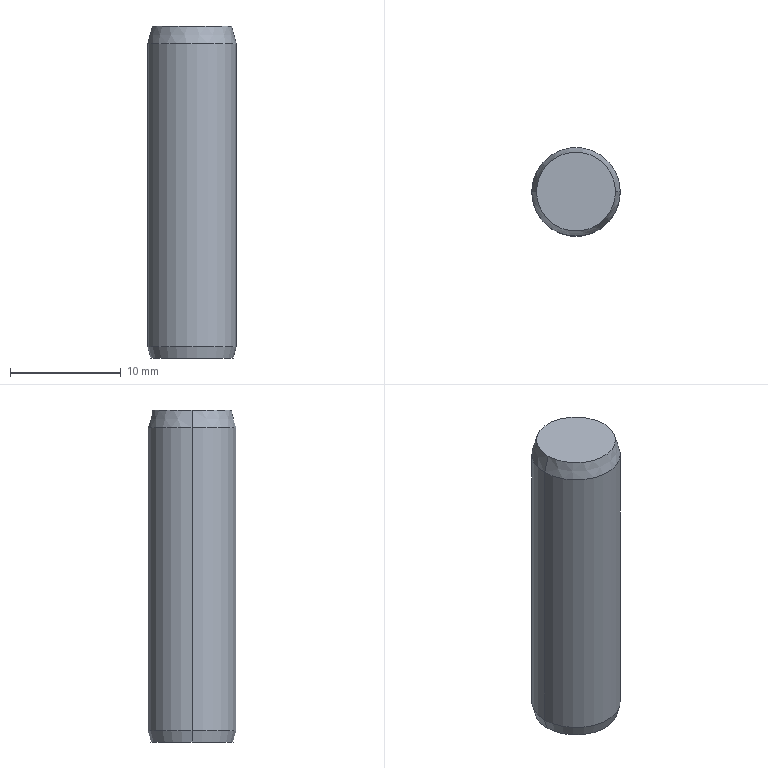Part | SolidWorks | features Chamfer 3, Cut 2, Extrusion 1, RevCut 1 | 1 solid | 16 faces | box 8 x 8 x 30 mm | volume 1303 mm3 | cone 8 | cylinder 6 | plane 2 | commonest cylinder face diameters 4.33 x2 5.3 x2 8 x2
STEP:
#1=CARTESIAN_POINT('',(2.165,0.,1.685));
#2=VERTEX_POINT('',#1);
#3=CARTESIAN_POINT('',(-2.165,0.,1.685));
#4=VERTEX_POINT('',#3);
#5=CARTESIAN_POINT('',(0.,0.,1.685));
#6=DIRECTION('',(0.,0.,-1.));
#7=DIRECTION('',(-1.,0.,0.));
#8=AXIS2_PLACEMENT_3D('',#5,#6,#7);
#9=CIRCLE('',#8,2.165);
#10=EDGE_CURVE('',#2,#4,#9,.T.);
#11=ORIENTED_EDGE('',*,*,#10,.F.);
#12=CARTESIAN_POINT('',(2.65,0.,1.2));
#13=VERTEX_POINT('',#12);
#14=CARTESIAN_POINT('',(2.65,0.,1.2));
#15=DIRECTION('',(0.7071,0.,-0.7071));
#16=VECTOR('',#15,1000.);
#17=LINE('',#14,#16);
#18=EDGE_CURVE('',#2,#13,#17,.T.);
#19=ORIENTED_EDGE('',*,*,#18,.T.);
#20=CARTESIAN_POINT('',(-2.65,0.,1.2));
#21=VERTEX_POINT('',#20);
#22=CARTESIAN_POINT('',(0.,0.,1.2));
#23=DIRECTION('',(0.,0.,-1.));
#24=DIRECTION('',(-1.,0.,0.));
#25=AXIS2_PLACEMENT_3D('',#22,#23,#24);
#26=CIRCLE('',#25,2.65);
#27=EDGE_CURVE('',#13,#21,#26,.T.);
#28=ORIENTED_EDGE('',*,*,#27,.T.);
#29=CARTESIAN_POINT('',(-2.65,0.,1.2));
#30=DIRECTION('',(-0.7071,0.,-0.7071));
#31=VECTOR('',#30,1000.);
#32=LINE('',#29,#31);
#33=EDGE_CURVE('',#4,#21,#32,.T.);
#34=ORIENTED_EDGE('',*,*,#33,.F.);
#35=EDGE_LOOP('',(#11,#19,#28,#34));
#36=FACE_OUTER_BOUND('',#35,.T.);
#37=CARTESIAN_POINT('',(0.,0.,1.2));
#38=DIRECTION('',(0.,0.,-1.));
#39=DIRECTION('',(-1.,0.,0.));
#40=AXIS2_PLACEMENT_3D('',#37,#38,#39);
#41=CONICAL_SURFACE('',#40,2.65,0.7854);
#42=ADVANCED_FACE('',(#36),#41,.F.);
#43=CARTESIAN_POINT('',(-2.165,0.,12.));
#44=VERTEX_POINT('',#43);
#45=CARTESIAN_POINT('',(2.165,0.,12.));
#46=VERTEX_POINT('',#45);
#47=CARTESIAN_POINT('',(0.,0.,12.));
#48=DIRECTION('',(0.,0.,1.));
#49=DIRECTION('',(1.,0.,0.));
#50=AXIS2_PLACEMENT_3D('',#47,#48,#49);
#51=CIRCLE('',#50,2.165);
#52=EDGE_CURVE('',#44,#46,#51,.T.);
#53=ORIENTED_EDGE('',*,*,#52,.T.);
#54=CARTESIAN_POINT('',(2.165,0.,12.));
#55=DIRECTION('',(0.,0.,-1.));
#56=VECTOR('',#55,1000.);
#57=LINE('',#54,#56);
#58=EDGE_CURVE('',#46,#2,#57,.T.);
#59=ORIENTED_EDGE('',*,*,#58,.T.);
#60=ORIENTED_EDGE('',*,*,#10,.T.);
#61=CARTESIAN_POINT('',(-2.165,0.,12.));
#62=DIRECTION('',(0.,0.,-1.));
#63=VECTOR('',#62,1000.);
#64=LINE('',#61,#63);
#65=EDGE_CURVE('',#44,#4,#64,.T.);
#66=ORIENTED_EDGE('',*,*,#65,.F.);
#67=EDGE_LOOP('',(#53,#59,#60,#66));
#68=FACE_OUTER_BOUND('',#67,.T.);
#69=CARTESIAN_POINT('',(0.,0.,12.));
#70=DIRECTION('',(0.,0.,-1.));
#71=DIRECTION('',(-1.,0.,0.));
#72=AXIS2_PLACEMENT_3D('',#69,#70,#71);
#73=CYLINDRICAL_SURFACE('',#72,2.165);
#74=ADVANCED_FACE('',(#68),#73,.F.);
#75=CARTESIAN_POINT('',(0.,0.,13.25));
#76=VERTEX_POINT('',#75);
#77=CARTESIAN_POINT('',(-2.165,0.,12.));
#78=DIRECTION('',(-0.866,0.,-0.5));
#79=VECTOR('',#78,1000.);
#80=LINE('',#77,#79);
#81=EDGE_CURVE('',#76,#44,#80,.T.);
#82=ORIENTED_EDGE('',*,*,#81,.F.);
#83=CARTESIAN_POINT('',(2.165,0.,12.));
#84=DIRECTION('',(0.866,0.,-0.5));
#85=VECTOR('',#84,1000.);
#86=LINE('',#83,#85);
#87=EDGE_CURVE('',#76,#46,#86,.T.);
#88=ORIENTED_EDGE('',*,*,#87,.T.);
#89=ORIENTED_EDGE('',*,*,#52,.F.);
#90=EDGE_LOOP('',(#82,#88,#89));
#91=FACE_OUTER_BOUND('',#90,.T.);
#92=CARTESIAN_POINT('',(0.,0.,12.));
#93=DIRECTION('',(0.,0.,-1.));
#94=DIRECTION('',(-1.,0.,0.));
#95=AXIS2_PLACEMENT_3D('',#92,#93,#94);
#96=CONICAL_SURFACE('',#95,2.165,1.047);
#97=ADVANCED_FACE('',(#91),#96,.F.);
#98=ORIENTED_EDGE('',*,*,#27,.F.);
#99=CARTESIAN_POINT('',(2.65,0.,0.));
#100=VERTEX_POINT('',#99);
#101=CARTESIAN_POINT('',(2.65,0.,1.2));
#102=DIRECTION('',(0.,0.,-1.));
#103=VECTOR('',#102,1000.);
#104=LINE('',#101,#103);
#105=EDGE_CURVE('',#13,#100,#104,.T.);
#106=ORIENTED_EDGE('',*,*,#105,.T.);
#107=CARTESIAN_POINT('',(-2.65,0.,0.));
#108=VERTEX_POINT('',#107);
#109=CARTESIAN_POINT('',(0.,0.,0.));
#110=DIRECTION('',(0.,0.,-1.));
#111=DIRECTION('',(-1.,0.,0.));
#112=AXIS2_PLACEMENT_3D('',#109,#110,#111);
#113=CIRCLE('',#112,2.65);
#114=EDGE_CURVE('',#100,#108,#113,.T.);
#115=ORIENTED_EDGE('',*,*,#114,.T.);
#116=CARTESIAN_POINT('',(-2.65,0.,1.2));
#117=DIRECTION('',(0.,0.,-1.));
#118=VECTOR('',#117,1000.);
#119=LINE('',#116,#118);
#120=EDGE_CURVE('',#21,#108,#119,.T.);
#121=ORIENTED_EDGE('',*,*,#120,.F.);
#122=EDGE_LOOP('',(#98,#106,#115,#121));
#123=FACE_OUTER_BOUND('',#122,.T.);
#124=CARTESIAN_POINT('',(0.,0.,1.2));
#125=DIRECTION('',(0.,0.,-1.));
#126=DIRECTION('',(-1.,0.,0.));
#127=AXIS2_PLACEMENT_3D('',#124,#125,#126);
#128=CYLINDRICAL_SURFACE('',#127,2.65);
#129=ADVANCED_FACE('',(#123),#128,.F.);
#130=CARTESIAN_POINT('',(-3.732,0.,0.));
#131=VERTEX_POINT('',#130);
#132=CARTESIAN_POINT('',(3.732,0.,0.));
#133=VERTEX_POINT('',#132);
#134=CARTESIAN_POINT('',(0.,0.,0.));
#135=DIRECTION('',(0.,0.,-1.));
#136=DIRECTION('',(1.,0.,0.));
#137=AXIS2_PLACEMENT_3D('',#134,#135,#136);
#138=CIRCLE('',#137,3.732);
#139=EDGE_CURVE('',#131,#133,#138,.T.);
#140=ORIENTED_EDGE('',*,*,#139,.F.);
#141=CARTESIAN_POINT('',(-4.,0.,1.));
#142=VERTEX_POINT('',#141);
#143=CARTESIAN_POINT('',(-4.,0.,1.));
#144=DIRECTION('',(-0.2588,0.,0.9659));
#145=VECTOR('',#144,1000.);
#146=LINE('',#143,#145);
#147=EDGE_CURVE('',#131,#142,#146,.T.);
#148=ORIENTED_EDGE('',*,*,#147,.T.);
#149=CARTESIAN_POINT('',(4.,0.,1.));
#150=VERTEX_POINT('',#149);
#151=CARTESIAN_POINT('',(0.,0.,1.));
#152=DIRECTION('',(0.,0.,1.));
#153=DIRECTION('',(1.,0.,0.));
#154=AXIS2_PLACEMENT_3D('',#151,#152,#153);
#155=CIRCLE('',#154,4.);
#156=EDGE_CURVE('',#150,#142,#155,.T.);
#157=ORIENTED_EDGE('',*,*,#156,.F.);
#158=CARTESIAN_POINT('',(4.,0.,1.));
#159=DIRECTION('',(0.2588,0.,0.9659));
#160=VECTOR('',#159,1000.);
#161=LINE('',#158,#160);
#162=EDGE_CURVE('',#133,#150,#161,.T.);
#163=ORIENTED_EDGE('',*,*,#162,.F.);
#164=EDGE_LOOP('',(#140,#148,#157,#163));
#165=FACE_OUTER_BOUND('',#164,.T.);
#166=CARTESIAN_POINT('',(0.,0.,1.));
#167=DIRECTION('',(0.,0.,1.));
#168=DIRECTION('',(1.,0.,0.));
#169=AXIS2_PLACEMENT_3D('',#166,#167,#168);
#170=CONICAL_SURFACE('',#169,4.,0.2618);
#171=ADVANCED_FACE('',(#165),#170,.T.);
#172=CARTESIAN_POINT('',(3.571,0.,30.));
#173=VERTEX_POINT('',#172);
#174=CARTESIAN_POINT('',(-3.571,0.,30.));
#175=VERTEX_POINT('',#174);
#176=CARTESIAN_POINT('',(0.,0.,30.));
#177=DIRECTION('',(0.,0.,1.));
#178=DIRECTION('',(1.,0.,0.));
#179=AXIS2_PLACEMENT_3D('',#176,#177,#178);
#180=CIRCLE('',#179,3.571);
#181=EDGE_CURVE('',#173,#175,#180,.T.);
#182=ORIENTED_EDGE('',*,*,#181,.F.);
#183=CARTESIAN_POINT('',(4.,0.,28.4));
#184=VERTEX_POINT('',#183);
#185=CARTESIAN_POINT('',(3.571,0.,30.));
#186=DIRECTION('',(0.2588,0.,-0.9659));
#187=VECTOR('',#186,1000.);
#188=LINE('',#185,#187);
#189=EDGE_CURVE('',#173,#184,#188,.T.);
#190=ORIENTED_EDGE('',*,*,#189,.T.);
#191=CARTESIAN_POINT('',(-4.,0.,28.4));
#192=VERTEX_POINT('',#191);
#193=CARTESIAN_POINT('',(0.,0.,28.4));
#194=DIRECTION('',(0.,0.,-1.));
#195=DIRECTION('',(1.,0.,0.));
#196=AXIS2_PLACEMENT_3D('',#193,#194,#195);
#197=CIRCLE('',#196,4.);
#198=EDGE_CURVE('',#192,#184,#197,.T.);
#199=ORIENTED_EDGE('',*,*,#198,.F.);
#200=CARTESIAN_POINT('',(-3.571,0.,30.));
#201=DIRECTION('',(-0.2588,0.,-0.9659));
#202=VECTOR('',#201,1000.);
#203=LINE('',#200,#202);
#204=EDGE_CURVE('',#175,#192,#203,.T.);
#205=ORIENTED_EDGE('',*,*,#204,.F.);
#206=EDGE_LOOP('',(#182,#190,#199,#205));
#207=FACE_OUTER_BOUND('',#206,.T.);
#208=CARTESIAN_POINT('',(0.,0.,30.));
#209=DIRECTION('',(0.,0.,-1.));
#210=DIRECTION('',(-1.,0.,0.));
#211=AXIS2_PLACEMENT_3D('',#208,#209,#210);
#212=CONICAL_SURFACE('',#211,3.571,0.2618);
#213=ADVANCED_FACE('',(#207),#212,.T.);
#214=ORIENTED_EDGE('',*,*,#198,.T.);
#215=CARTESIAN_POINT('',(4.,0.,30.));
#216=DIRECTION('',(0.,0.,-1.));
#217=VECTOR('',#216,1000.);
#218=LINE('',#215,#217);
#219=EDGE_CURVE('',#184,#150,#218,.T.);
#220=ORIENTED_EDGE('',*,*,#219,.T.);
#221=ORIENTED_EDGE('',*,*,#156,.T.);
#222=CARTESIAN_POINT('',(-4.,0.,30.));
#223=DIRECTION('',(0.,0.,-1.));
#224=VECTOR('',#223,1000.);
#225=LINE('',#222,#224);
#226=EDGE_CURVE('',#192,#142,#225,.T.);
#227=ORIENTED_EDGE('',*,*,#226,.F.);
#228=EDGE_LOOP('',(#214,#220,#221,#227));
#229=FACE_OUTER_BOUND('',#228,.T.);
#230=CARTESIAN_POINT('',(0.,0.,30.));
#231=DIRECTION('',(0.,0.,-1.));
#232=DIRECTION('',(-1.,0.,0.));
#233=AXIS2_PLACEMENT_3D('',#230,#231,#232);
#234=CYLINDRICAL_SURFACE('',#233,4.);
#235=ADVANCED_FACE('',(#229),#234,.T.);
#236=ORIENTED_EDGE('',*,*,#219,.F.);
#237=CARTESIAN_POINT('',(0.,0.,28.4));
#238=DIRECTION('',(0.,0.,-1.));
#239=DIRECTION('',(1.,0.,0.));
#240=AXIS2_PLACEMENT_3D('',#237,#238,#239);
#241=CIRCLE('',#240,4.);
#242=EDGE_CURVE('',#184,#192,#241,.T.);
#243=ORIENTED_EDGE('',*,*,#242,.T.);
#244=ORIENTED_EDGE('',*,*,#226,.T.);
#245=CARTESIAN_POINT('',(0.,0.,1.));
#246=DIRECTION('',(0.,0.,1.));
#247=DIRECTION('',(1.,0.,0.));
#248=AXIS2_PLACEMENT_3D('',#245,#246,#247);
#249=CIRCLE('',#248,4.);
#250=EDGE_CURVE('',#142,#150,#249,.T.);
#251=ORIENTED_EDGE('',*,*,#250,.T.);
#252=EDGE_LOOP('',(#236,#243,#244,#251));
#253=FACE_OUTER_BOUND('',#252,.T.);
#254=CARTESIAN_POINT('',(0.,0.,30.));
#255=DIRECTION('',(0.,0.,-1.));
#256=DIRECTION('',(-1.,0.,0.));
#257=AXIS2_PLACEMENT_3D('',#254,#255,#256);
#258=CYLINDRICAL_SURFACE('',#257,4.);
#259=ADVANCED_FACE('',(#253),#258,.T.);
#260=CARTESIAN_POINT('',(0.,0.,30.));
#261=DIRECTION('',(0.,0.,1.));
#262=DIRECTION('',(1.,0.,0.));
#263=AXIS2_PLACEMENT_3D('',#260,#261,#262);
#264=CIRCLE('',#263,3.571);
#265=EDGE_CURVE('',#175,#173,#264,.T.);
#266=ORIENTED_EDGE('',*,*,#265,.T.);
#267=ORIENTED_EDGE('',*,*,#181,.T.);
#268=EDGE_LOOP('',(#266,#267));
#269=FACE_OUTER_BOUND('',#268,.T.);
#270=CARTESIAN_POINT('',(0.,0.,30.));
#271=DIRECTION('',(0.,0.,1.));
#272=DIRECTION('',(1.,0.,0.));
#273=AXIS2_PLACEMENT_3D('',#270,#271,#272);
#274=PLANE('',#273);
#275=ADVANCED_FACE('',(#269),#274,.T.);
#276=CARTESIAN_POINT('',(0.,0.,0.));
#277=DIRECTION('',(0.,0.,-1.));
#278=DIRECTION('',(-1.,0.,0.));
#279=AXIS2_PLACEMENT_3D('',#276,#277,#278);
#280=CIRCLE('',#279,2.65);
#281=EDGE_CURVE('',#108,#100,#280,.T.);
#282=ORIENTED_EDGE('',*,*,#281,.F.);
#283=ORIENTED_EDGE('',*,*,#114,.F.);
#284=EDGE_LOOP('',(#282,#283));
#285=FACE_BOUND('',#284,.T.);
#286=CARTESIAN_POINT('',(0.,0.,0.));
#287=DIRECTION('',(0.,0.,-1.));
#288=DIRECTION('',(1.,0.,0.));
#289=AXIS2_PLACEMENT_3D('',#286,#287,#288);
#290=CIRCLE('',#289,3.732);
#291=EDGE_CURVE('',#133,#131,#290,.T.);
#292=ORIENTED_EDGE('',*,*,#291,.T.);
#293=ORIENTED_EDGE('',*,*,#139,.T.);
#294=EDGE_LOOP('',(#292,#293));
#295=FACE_OUTER_BOUND('',#294,.T.);
#296=CARTESIAN_POINT('',(0.,0.,0.));
#297=DIRECTION('',(0.,0.,1.));
#298=DIRECTION('',(1.,0.,0.));
#299=AXIS2_PLACEMENT_3D('',#296,#297,#298);
#300=PLANE('',#299);
#301=ADVANCED_FACE('',(#285,#295),#300,.F.);
#302=ORIENTED_EDGE('',*,*,#189,.F.);
#303=ORIENTED_EDGE('',*,*,#265,.F.);
#304=ORIENTED_EDGE('',*,*,#204,.T.);
#305=ORIENTED_EDGE('',*,*,#242,.F.);
#306=EDGE_LOOP('',(#302,#303,#304,#305));
#307=FACE_OUTER_BOUND('',#306,.T.);
#308=CARTESIAN_POINT('',(0.,0.,30.));
#309=DIRECTION('',(0.,0.,-1.));
#310=DIRECTION('',(-1.,0.,0.));
#311=AXIS2_PLACEMENT_3D('',#308,#309,#310);
#312=CONICAL_SURFACE('',#311,3.571,0.2618);
#313=ADVANCED_FACE('',(#307),#312,.T.);
#314=ORIENTED_EDGE('',*,*,#147,.F.);
#315=ORIENTED_EDGE('',*,*,#291,.F.);
#316=ORIENTED_EDGE('',*,*,#162,.T.);
#317=ORIENTED_EDGE('',*,*,#250,.F.);
#318=EDGE_LOOP('',(#314,#315,#316,#317));
#319=FACE_OUTER_BOUND('',#318,.T.);
#320=CARTESIAN_POINT('',(0.,0.,1.));
#321=DIRECTION('',(0.,0.,1.));
#322=DIRECTION('',(1.,0.,0.));
#323=AXIS2_PLACEMENT_3D('',#320,#321,#322);
#324=CONICAL_SURFACE('',#323,4.,0.2618);
#325=ADVANCED_FACE('',(#319),#324,.T.);
#326=ORIENTED_EDGE('',*,*,#105,.F.);
#327=CARTESIAN_POINT('',(0.,0.,1.2));
#328=DIRECTION('',(0.,0.,-1.));
#329=DIRECTION('',(-1.,0.,0.));
#330=AXIS2_PLACEMENT_3D('',#327,#328,#329);
#331=CIRCLE('',#330,2.65);
#332=EDGE_CURVE('',#21,#13,#331,.T.);
#333=ORIENTED_EDGE('',*,*,#332,.F.);
#334=ORIENTED_EDGE('',*,*,#120,.T.);
#335=ORIENTED_EDGE('',*,*,#281,.T.);
#336=EDGE_LOOP('',(#326,#333,#334,#335));
#337=FACE_OUTER_BOUND('',#336,.T.);
#338=CARTESIAN_POINT('',(0.,0.,1.2));
#339=DIRECTION('',(0.,0.,-1.));
#340=DIRECTION('',(-1.,0.,0.));
#341=AXIS2_PLACEMENT_3D('',#338,#339,#340);
#342=CYLINDRICAL_SURFACE('',#341,2.65);
#343=ADVANCED_FACE('',(#337),#342,.F.);
#344=ORIENTED_EDGE('',*,*,#87,.F.);
#345=ORIENTED_EDGE('',*,*,#81,.T.);
#346=CARTESIAN_POINT('',(0.,0.,12.));
#347=DIRECTION('',(0.,0.,1.));
#348=DIRECTION('',(1.,0.,0.));
#349=AXIS2_PLACEMENT_3D('',#346,#347,#348);
#350=CIRCLE('',#349,2.165);
#351=EDGE_CURVE('',#46,#44,#350,.T.);
#352=ORIENTED_EDGE('',*,*,#351,.F.);
#353=EDGE_LOOP('',(#344,#345,#352));
#354=FACE_OUTER_BOUND('',#353,.T.);
#355=CARTESIAN_POINT('',(0.,0.,12.));
#356=DIRECTION('',(0.,0.,-1.));
#357=DIRECTION('',(-1.,0.,0.));
#358=AXIS2_PLACEMENT_3D('',#355,#356,#357);
#359=CONICAL_SURFACE('',#358,2.165,1.047);
#360=ADVANCED_FACE('',(#354),#359,.F.);
#361=ORIENTED_EDGE('',*,*,#58,.F.);
#362=ORIENTED_EDGE('',*,*,#351,.T.);
#363=ORIENTED_EDGE('',*,*,#65,.T.);
#364=CARTESIAN_POINT('',(0.,0.,1.685));
#365=DIRECTION('',(0.,0.,-1.));
#366=DIRECTION('',(-1.,0.,0.));
#367=AXIS2_PLACEMENT_3D('',#364,#365,#366);
#368=CIRCLE('',#367,2.165);
#369=EDGE_CURVE('',#4,#2,#368,.T.);
#370=ORIENTED_EDGE('',*,*,#369,.T.);
#371=EDGE_LOOP('',(#361,#362,#363,#370));
#372=FACE_OUTER_BOUND('',#371,.T.);
#373=CARTESIAN_POINT('',(0.,0.,12.));
#374=DIRECTION('',(0.,0.,-1.));
#375=DIRECTION('',(-1.,0.,0.));
#376=AXIS2_PLACEMENT_3D('',#373,#374,#375);
#377=CYLINDRICAL_SURFACE('',#376,2.165);
#378=ADVANCED_FACE('',(#372),#377,.F.);
#379=ORIENTED_EDGE('',*,*,#18,.F.);
#380=ORIENTED_EDGE('',*,*,#369,.F.);
#381=ORIENTED_EDGE('',*,*,#33,.T.);
#382=ORIENTED_EDGE('',*,*,#332,.T.);
#383=EDGE_LOOP('',(#379,#380,#381,#382));
#384=FACE_OUTER_BOUND('',#383,.T.);
#385=CARTESIAN_POINT('',(0.,0.,1.2));
#386=DIRECTION('',(0.,0.,-1.));
#387=DIRECTION('',(-1.,0.,0.));
#388=AXIS2_PLACEMENT_3D('',#385,#386,#387);
#389=CONICAL_SURFACE('',#388,2.65,0.7854);
#390=ADVANCED_FACE('',(#384),#389,.F.);
#391=CLOSED_SHELL('',(#42,#74,#97,#129,#171,#213,#235,#259,#275,#301,#313,#325,#343,#360,#378,#390));
#392=MANIFOLD_SOLID_BREP('',#391);
#393=CARTESIAN_POINT('',(0.,0.,0.));
#394=DIRECTION('',(0.,0.,1.));
#395=DIRECTION('',(1.,0.,0.));
#396=AXIS2_PLACEMENT_3D('',#393,#394,#395);
#397=(LENGTH_UNIT()NAMED_UNIT(*)SI_UNIT(.MILLI.,.METRE.));
#398=UNCERTAINTY_MEASURE_WITH_UNIT(LENGTH_MEASURE(0.00001),#397,'','');
#399=(NAMED_UNIT(*)PLANE_ANGLE_UNIT()SI_UNIT($,.RADIAN.));
#400=(NAMED_UNIT(*)SI_UNIT($,.STERADIAN.)SOLID_ANGLE_UNIT());
#401=(GEOMETRIC_REPRESENTATION_CONTEXT(3)GLOBAL_UNCERTAINTY_ASSIGNED_CONTEXT((#398))GLOBAL_UNIT_ASSIGNED_CONTEXT((#397,#399,#400))REPRESENTATION_CONTEXT('',''));
#402=ADVANCED_BREP_SHAPE_REPRESENTATION('',(#392,#396),#401);